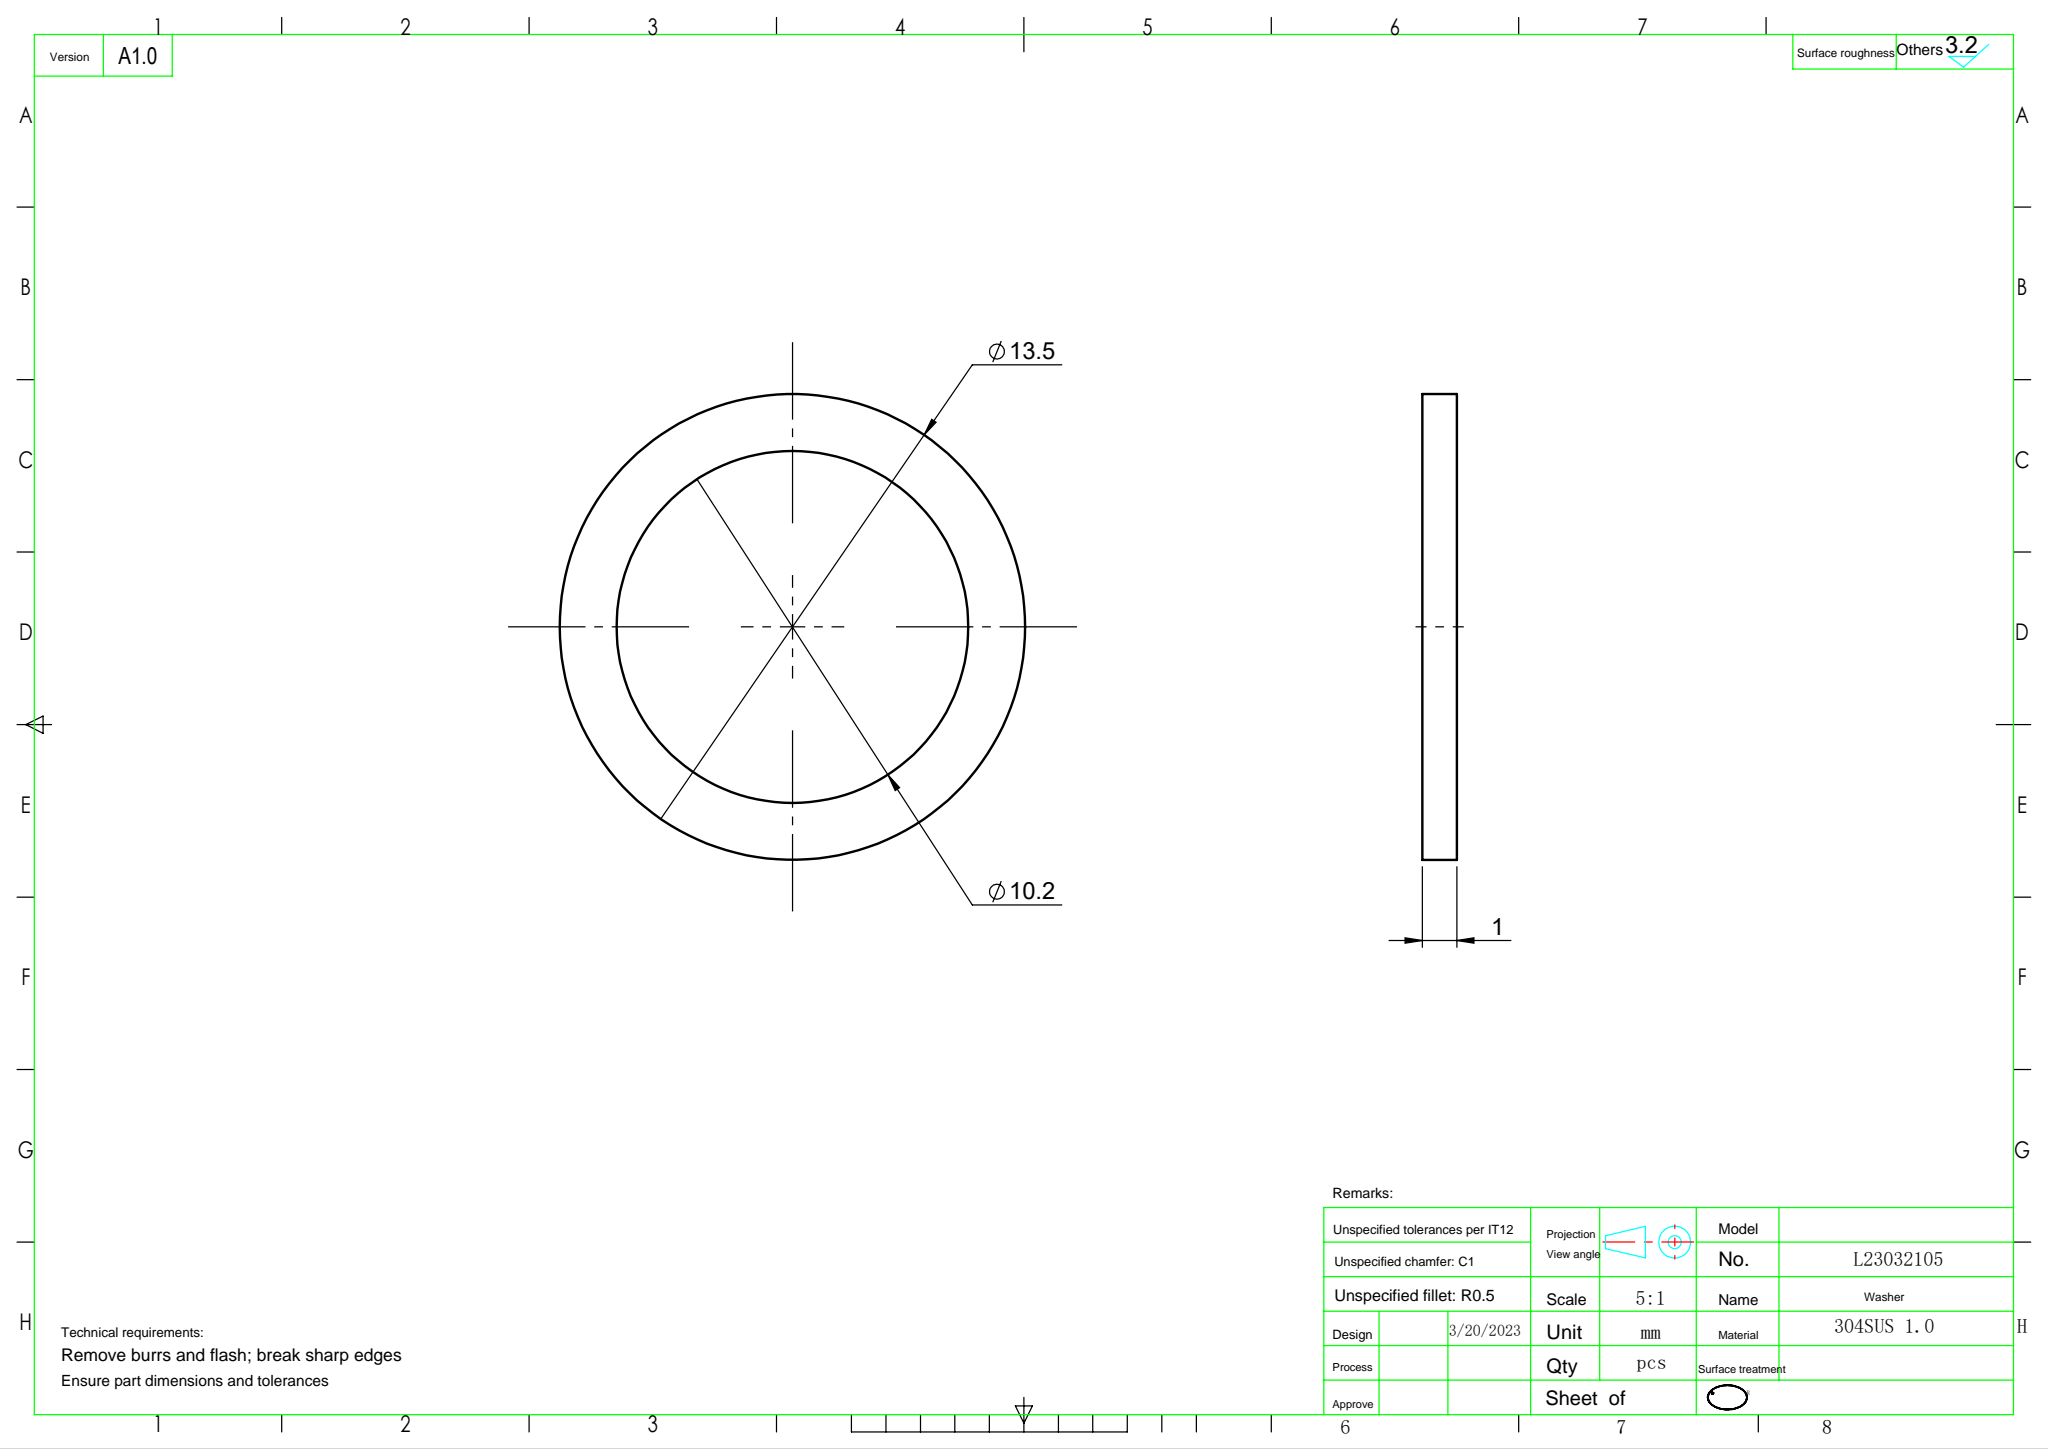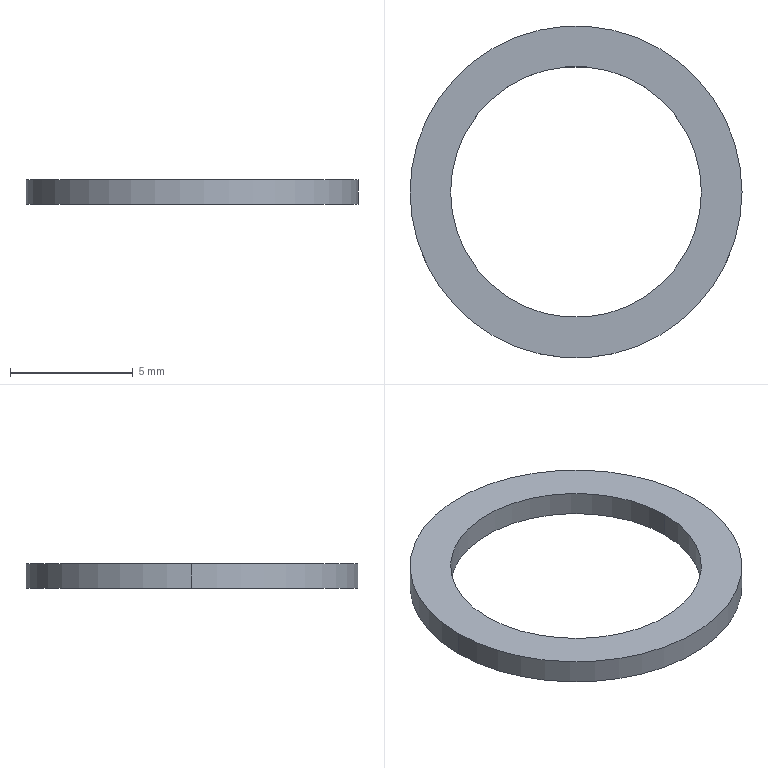Part | SolidWorks | features FlatPattern 1, SMBaseFlange 1, SheetMetal 1 | 1 solid | 6 faces | box 13.5 x 13.5 x 1 mm | volume 61.426 mm3 | cylinder 4 | plane 2 | commonest cylinder face diameters 10.2 x2 13.5 x2
STEP:
#1=CARTESIAN_POINT('',(-5.1,0.,-1.));
#2=VERTEX_POINT('',#1);
#3=CARTESIAN_POINT('',(5.1,0.,-1.));
#4=VERTEX_POINT('',#3);
#5=CARTESIAN_POINT('',(0.,0.,-1.));
#6=DIRECTION('',(0.,0.,1.));
#7=DIRECTION('',(1.,0.,0.));
#8=AXIS2_PLACEMENT_3D('',#5,#6,#7);
#9=CIRCLE('',#8,5.1);
#10=EDGE_CURVE('',#2,#4,#9,.T.);
#11=ORIENTED_EDGE('',*,*,#10,.F.);
#12=CARTESIAN_POINT('',(-5.1,0.,0.));
#13=VERTEX_POINT('',#12);
#14=CARTESIAN_POINT('',(-5.1,0.,-1.));
#15=DIRECTION('',(0.,0.,1.));
#16=VECTOR('',#15,1000.);
#17=LINE('',#14,#16);
#18=EDGE_CURVE('',#2,#13,#17,.T.);
#19=ORIENTED_EDGE('',*,*,#18,.T.);
#20=CARTESIAN_POINT('',(5.1,0.,0.));
#21=VERTEX_POINT('',#20);
#22=CARTESIAN_POINT('',(0.,0.,0.));
#23=DIRECTION('',(0.,0.,1.));
#24=DIRECTION('',(1.,0.,0.));
#25=AXIS2_PLACEMENT_3D('',#22,#23,#24);
#26=CIRCLE('',#25,5.1);
#27=EDGE_CURVE('',#13,#21,#26,.T.);
#28=ORIENTED_EDGE('',*,*,#27,.T.);
#29=CARTESIAN_POINT('',(5.1,0.,-1.));
#30=DIRECTION('',(0.,0.,1.));
#31=VECTOR('',#30,1000.);
#32=LINE('',#29,#31);
#33=EDGE_CURVE('',#4,#21,#32,.T.);
#34=ORIENTED_EDGE('',*,*,#33,.F.);
#35=EDGE_LOOP('',(#11,#19,#28,#34));
#36=FACE_OUTER_BOUND('',#35,.T.);
#37=CARTESIAN_POINT('',(0.,0.,-1.));
#38=DIRECTION('',(0.,0.,1.));
#39=DIRECTION('',(1.,0.,0.));
#40=AXIS2_PLACEMENT_3D('',#37,#38,#39);
#41=CYLINDRICAL_SURFACE('',#40,5.1);
#42=ADVANCED_FACE('',(#36),#41,.F.);
#43=CARTESIAN_POINT('',(6.75,0.,-1.));
#44=VERTEX_POINT('',#43);
#45=CARTESIAN_POINT('',(-6.75,0.,-1.));
#46=VERTEX_POINT('',#45);
#47=CARTESIAN_POINT('',(0.,0.,-1.));
#48=DIRECTION('',(0.,0.,1.));
#49=DIRECTION('',(1.,0.,0.));
#50=AXIS2_PLACEMENT_3D('',#47,#48,#49);
#51=CIRCLE('',#50,6.75);
#52=EDGE_CURVE('',#44,#46,#51,.T.);
#53=ORIENTED_EDGE('',*,*,#52,.T.);
#54=CARTESIAN_POINT('',(-6.75,0.,0.));
#55=VERTEX_POINT('',#54);
#56=CARTESIAN_POINT('',(-6.75,0.,-1.));
#57=DIRECTION('',(0.,0.,1.));
#58=VECTOR('',#57,1000.);
#59=LINE('',#56,#58);
#60=EDGE_CURVE('',#46,#55,#59,.T.);
#61=ORIENTED_EDGE('',*,*,#60,.T.);
#62=CARTESIAN_POINT('',(6.75,0.,0.));
#63=VERTEX_POINT('',#62);
#64=CARTESIAN_POINT('',(0.,0.,0.));
#65=DIRECTION('',(0.,0.,1.));
#66=DIRECTION('',(1.,0.,0.));
#67=AXIS2_PLACEMENT_3D('',#64,#65,#66);
#68=CIRCLE('',#67,6.75);
#69=EDGE_CURVE('',#63,#55,#68,.T.);
#70=ORIENTED_EDGE('',*,*,#69,.F.);
#71=CARTESIAN_POINT('',(6.75,0.,-1.));
#72=DIRECTION('',(0.,0.,1.));
#73=VECTOR('',#72,1000.);
#74=LINE('',#71,#73);
#75=EDGE_CURVE('',#44,#63,#74,.T.);
#76=ORIENTED_EDGE('',*,*,#75,.F.);
#77=EDGE_LOOP('',(#53,#61,#70,#76));
#78=FACE_OUTER_BOUND('',#77,.T.);
#79=CARTESIAN_POINT('',(0.,0.,-1.));
#80=DIRECTION('',(0.,0.,1.));
#81=DIRECTION('',(1.,0.,0.));
#82=AXIS2_PLACEMENT_3D('',#79,#80,#81);
#83=CYLINDRICAL_SURFACE('',#82,6.75);
#84=ADVANCED_FACE('',(#78),#83,.T.);
#85=ORIENTED_EDGE('',*,*,#60,.F.);
#86=CARTESIAN_POINT('',(0.,0.,-1.));
#87=DIRECTION('',(0.,0.,1.));
#88=DIRECTION('',(1.,0.,0.));
#89=AXIS2_PLACEMENT_3D('',#86,#87,#88);
#90=CIRCLE('',#89,6.75);
#91=EDGE_CURVE('',#46,#44,#90,.T.);
#92=ORIENTED_EDGE('',*,*,#91,.T.);
#93=ORIENTED_EDGE('',*,*,#75,.T.);
#94=CARTESIAN_POINT('',(0.,0.,0.));
#95=DIRECTION('',(0.,0.,1.));
#96=DIRECTION('',(1.,0.,0.));
#97=AXIS2_PLACEMENT_3D('',#94,#95,#96);
#98=CIRCLE('',#97,6.75);
#99=EDGE_CURVE('',#55,#63,#98,.T.);
#100=ORIENTED_EDGE('',*,*,#99,.F.);
#101=EDGE_LOOP('',(#85,#92,#93,#100));
#102=FACE_OUTER_BOUND('',#101,.T.);
#103=CARTESIAN_POINT('',(0.,0.,-1.));
#104=DIRECTION('',(0.,0.,1.));
#105=DIRECTION('',(1.,0.,0.));
#106=AXIS2_PLACEMENT_3D('',#103,#104,#105);
#107=CYLINDRICAL_SURFACE('',#106,6.75);
#108=ADVANCED_FACE('',(#102),#107,.T.);
#109=CARTESIAN_POINT('',(0.,0.,-1.));
#110=DIRECTION('',(0.,0.,1.));
#111=DIRECTION('',(1.,0.,0.));
#112=AXIS2_PLACEMENT_3D('',#109,#110,#111);
#113=CIRCLE('',#112,5.1);
#114=EDGE_CURVE('',#4,#2,#113,.T.);
#115=ORIENTED_EDGE('',*,*,#114,.T.);
#116=ORIENTED_EDGE('',*,*,#10,.T.);
#117=EDGE_LOOP('',(#115,#116));
#118=FACE_BOUND('',#117,.T.);
#119=ORIENTED_EDGE('',*,*,#52,.F.);
#120=ORIENTED_EDGE('',*,*,#91,.F.);
#121=EDGE_LOOP('',(#119,#120));
#122=FACE_OUTER_BOUND('',#121,.T.);
#123=CARTESIAN_POINT('',(0.,0.,-1.));
#124=DIRECTION('',(0.,0.,1.));
#125=DIRECTION('',(1.,0.,0.));
#126=AXIS2_PLACEMENT_3D('',#123,#124,#125);
#127=PLANE('',#126);
#128=ADVANCED_FACE('',(#118,#122),#127,.F.);
#129=CARTESIAN_POINT('',(0.,0.,0.));
#130=DIRECTION('',(0.,0.,1.));
#131=DIRECTION('',(1.,0.,0.));
#132=AXIS2_PLACEMENT_3D('',#129,#130,#131);
#133=CIRCLE('',#132,5.1);
#134=EDGE_CURVE('',#21,#13,#133,.T.);
#135=ORIENTED_EDGE('',*,*,#134,.F.);
#136=ORIENTED_EDGE('',*,*,#27,.F.);
#137=EDGE_LOOP('',(#135,#136));
#138=FACE_BOUND('',#137,.T.);
#139=ORIENTED_EDGE('',*,*,#69,.T.);
#140=ORIENTED_EDGE('',*,*,#99,.T.);
#141=EDGE_LOOP('',(#139,#140));
#142=FACE_OUTER_BOUND('',#141,.T.);
#143=CARTESIAN_POINT('',(0.,0.,0.));
#144=DIRECTION('',(0.,0.,1.));
#145=DIRECTION('',(1.,0.,0.));
#146=AXIS2_PLACEMENT_3D('',#143,#144,#145);
#147=PLANE('',#146);
#148=ADVANCED_FACE('',(#138,#142),#147,.T.);
#149=ORIENTED_EDGE('',*,*,#18,.F.);
#150=ORIENTED_EDGE('',*,*,#114,.F.);
#151=ORIENTED_EDGE('',*,*,#33,.T.);
#152=ORIENTED_EDGE('',*,*,#134,.T.);
#153=EDGE_LOOP('',(#149,#150,#151,#152));
#154=FACE_OUTER_BOUND('',#153,.T.);
#155=CARTESIAN_POINT('',(0.,0.,-1.));
#156=DIRECTION('',(0.,0.,1.));
#157=DIRECTION('',(1.,0.,0.));
#158=AXIS2_PLACEMENT_3D('',#155,#156,#157);
#159=CYLINDRICAL_SURFACE('',#158,5.1);
#160=ADVANCED_FACE('',(#154),#159,.F.);
#161=CLOSED_SHELL('',(#42,#84,#108,#128,#148,#160));
#162=MANIFOLD_SOLID_BREP('',#161);
#163=CARTESIAN_POINT('',(0.,0.,0.));
#164=DIRECTION('',(0.,0.,1.));
#165=DIRECTION('',(1.,0.,0.));
#166=AXIS2_PLACEMENT_3D('',#163,#164,#165);
#167=(LENGTH_UNIT()NAMED_UNIT(*)SI_UNIT(.MILLI.,.METRE.));
#168=UNCERTAINTY_MEASURE_WITH_UNIT(LENGTH_MEASURE(0.00001),#167,'','');
#169=(NAMED_UNIT(*)PLANE_ANGLE_UNIT()SI_UNIT($,.RADIAN.));
#170=(NAMED_UNIT(*)SI_UNIT($,.STERADIAN.)SOLID_ANGLE_UNIT());
#171=(GEOMETRIC_REPRESENTATION_CONTEXT(3)GLOBAL_UNCERTAINTY_ASSIGNED_CONTEXT((#168))GLOBAL_UNIT_ASSIGNED_CONTEXT((#167,#169,#170))REPRESENTATION_CONTEXT('',''));
#172=ADVANCED_BREP_SHAPE_REPRESENTATION('',(#162,#166),#171);